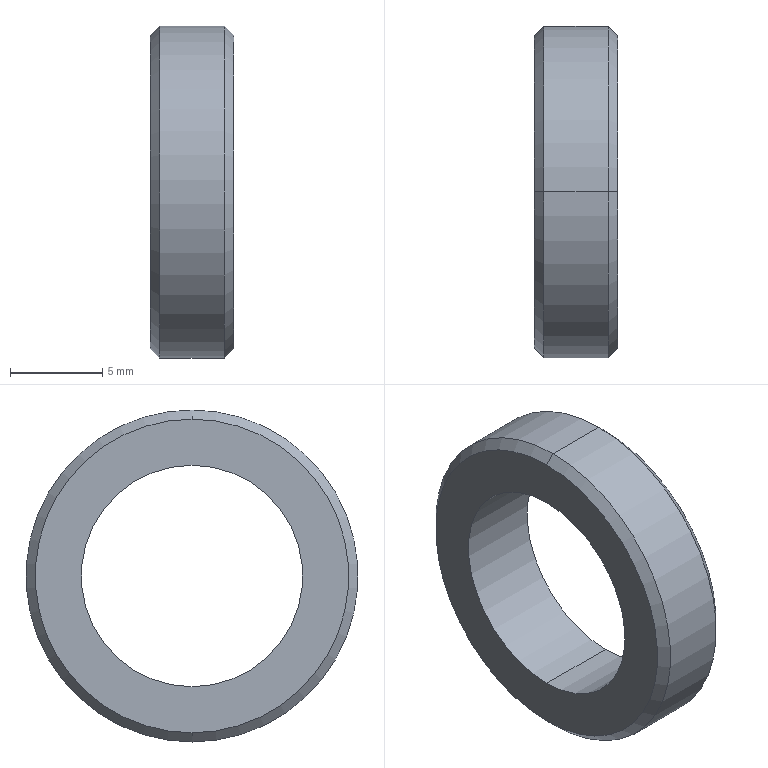Part | STEP file | 0245_008_CLBUM12-18-4.5 | 1 solid | 10 faces | box 4.5 x 18 x 18 mm | volume 622.297 mm3 | cone 4 | cylinder 4 | plane 2 | commonest cylinder face diameters 12 x2 18 x2
STEP:
#1=CARTESIAN_POINT('',(0.,0.,0.));
#2=DIRECTION('',(0.,0.,1.));
#3=DIRECTION('',(1.,0.,0.));
#4=AXIS2_PLACEMENT_3D('',#1,#2,#3);
#5=CARTESIAN_POINT('',(0.,0.,8.5));
#6=VERTEX_POINT('',#5);
#7=CARTESIAN_POINT('',(0.,0.,-8.5));
#8=VERTEX_POINT('',#7);
#9=CARTESIAN_POINT('',(0.,0.,0.));
#10=DIRECTION('',(-1.,0.,0.));
#11=DIRECTION('',(0.,0.,-1.));
#12=AXIS2_PLACEMENT_3D('',#9,#10,#11);
#13=CIRCLE('',#12,8.5);
#14=CARTESIAN_POINT('',(0.5,0.,0.));
#15=DIRECTION('',(1.,0.,0.));
#16=DIRECTION('',(0.,0.,-1.));
#17=AXIS2_PLACEMENT_3D('',#14,#15,#16);
#18=CONICAL_SURFACE('',#17,9.,0.7854);
#19=CARTESIAN_POINT('',(6.283,-0.5));
#20=DIRECTION('',(-1.,0.));
#21=VECTOR('',#20,1.);
#22=LINE('',#19,#21);
#23=(GEOMETRIC_REPRESENTATION_CONTEXT(2)PARAMETRIC_REPRESENTATION_CONTEXT()REPRESENTATION_CONTEXT('',''));
#24=DEFINITIONAL_REPRESENTATION('',(#22),#23);
#25=PCURVE('',#18,#24);
#26=CARTESIAN_POINT('',(0.,7.25,0.));
#27=DIRECTION('',(-1.,0.,0.));
#28=DIRECTION('',(0.,0.,1.));
#29=AXIS2_PLACEMENT_3D('',#26,#27,#28);
#30=PLANE('',#29);
#31=CARTESIAN_POINT('',(0.,-7.25));
#32=DIRECTION('',(-1.,0.));
#33=AXIS2_PLACEMENT_2D('',#31,#32);
#34=CIRCLE('',#33,8.5);
#35=(GEOMETRIC_REPRESENTATION_CONTEXT(2)PARAMETRIC_REPRESENTATION_CONTEXT()REPRESENTATION_CONTEXT('',''));
#36=DEFINITIONAL_REPRESENTATION('',(#34),#35);
#37=PCURVE('',#30,#36);
#38=SURFACE_CURVE('',#13,(#25,#37),.PCURVE_S1.);
#39=EDGE_CURVE('',#6,#8,#38,.T.);
#40=ORIENTED_EDGE('',*,*,#39,.F.);
#41=CARTESIAN_POINT('',(0.5,0.,9.));
#42=VERTEX_POINT('',#41);
#43=CARTESIAN_POINT('',(0.5,0.,9.));
#44=DIRECTION('',(0.7071,0.,0.7071));
#45=VECTOR('',#44,1.);
#46=LINE('',#43,#45);
#47=CARTESIAN_POINT('',(3.142,0.));
#48=DIRECTION('',(0.,1.));
#49=VECTOR('',#48,1.);
#50=LINE('',#47,#49);
#51=(GEOMETRIC_REPRESENTATION_CONTEXT(2)PARAMETRIC_REPRESENTATION_CONTEXT()REPRESENTATION_CONTEXT('',''));
#52=DEFINITIONAL_REPRESENTATION('',(#50),#51);
#53=PCURVE('',#18,#52);
#54=CARTESIAN_POINT('',(0.5,0.,0.));
#55=DIRECTION('',(1.,0.,0.));
#56=DIRECTION('',(0.,0.,-1.));
#57=AXIS2_PLACEMENT_3D('',#54,#55,#56);
#58=CONICAL_SURFACE('',#57,9.,0.7854);
#59=CARTESIAN_POINT('',(3.142,0.));
#60=DIRECTION('',(0.,1.));
#61=VECTOR('',#60,1.);
#62=LINE('',#59,#61);
#63=(GEOMETRIC_REPRESENTATION_CONTEXT(2)PARAMETRIC_REPRESENTATION_CONTEXT()REPRESENTATION_CONTEXT('',''));
#64=DEFINITIONAL_REPRESENTATION('',(#62),#63);
#65=PCURVE('',#58,#64);
#66=SURFACE_CURVE('',#46,(#53,#65),.PCURVE_S1.);
#67=EDGE_CURVE('',#6,#42,#66,.T.);
#68=ORIENTED_EDGE('',*,*,#67,.T.);
#69=CARTESIAN_POINT('',(0.5,0.,-9.));
#70=VERTEX_POINT('',#69);
#71=CARTESIAN_POINT('',(0.5,0.,0.));
#72=DIRECTION('',(-1.,0.,0.));
#73=DIRECTION('',(0.,1.,0.));
#74=AXIS2_PLACEMENT_3D('',#71,#72,#73);
#75=CIRCLE('',#74,9.);
#76=CARTESIAN_POINT('',(7.854,0.));
#77=DIRECTION('',(-1.,0.));
#78=VECTOR('',#77,1.);
#79=LINE('',#76,#78);
#80=(GEOMETRIC_REPRESENTATION_CONTEXT(2)PARAMETRIC_REPRESENTATION_CONTEXT()REPRESENTATION_CONTEXT('',''));
#81=DEFINITIONAL_REPRESENTATION('',(#79),#80);
#82=PCURVE('',#18,#81);
#83=CARTESIAN_POINT('',(2.25,0.,0.));
#84=DIRECTION('',(1.,0.,0.));
#85=DIRECTION('',(0.,0.,-1.));
#86=AXIS2_PLACEMENT_3D('',#83,#84,#85);
#87=CYLINDRICAL_SURFACE('',#86,9.);
#88=CARTESIAN_POINT('',(7.854,-1.75));
#89=DIRECTION('',(-1.,0.));
#90=VECTOR('',#89,1.);
#91=LINE('',#88,#90);
#92=(GEOMETRIC_REPRESENTATION_CONTEXT(2)PARAMETRIC_REPRESENTATION_CONTEXT()REPRESENTATION_CONTEXT('',''));
#93=DEFINITIONAL_REPRESENTATION('',(#91),#92);
#94=PCURVE('',#87,#93);
#95=SURFACE_CURVE('',#75,(#82,#94),.PCURVE_S1.);
#96=EDGE_CURVE('',#42,#70,#95,.T.);
#97=ORIENTED_EDGE('',*,*,#96,.T.);
#98=CARTESIAN_POINT('',(0.5,0.,-9.));
#99=DIRECTION('',(0.7071,0.,-0.7071));
#100=VECTOR('',#99,1.);
#101=LINE('',#98,#100);
#102=CARTESIAN_POINT('',(0.,0.));
#103=DIRECTION('',(0.,1.));
#104=VECTOR('',#103,1.);
#105=LINE('',#102,#104);
#106=(GEOMETRIC_REPRESENTATION_CONTEXT(2)PARAMETRIC_REPRESENTATION_CONTEXT()REPRESENTATION_CONTEXT('',''));
#107=DEFINITIONAL_REPRESENTATION('',(#105),#106);
#108=PCURVE('',#18,#107);
#109=CARTESIAN_POINT('',(6.283,0.));
#110=DIRECTION('',(0.,1.));
#111=VECTOR('',#110,1.);
#112=LINE('',#109,#111);
#113=(GEOMETRIC_REPRESENTATION_CONTEXT(2)PARAMETRIC_REPRESENTATION_CONTEXT()REPRESENTATION_CONTEXT('',''));
#114=DEFINITIONAL_REPRESENTATION('',(#112),#113);
#115=PCURVE('',#58,#114);
#116=SURFACE_CURVE('',#101,(#108,#115),.PCURVE_S1.);
#117=EDGE_CURVE('',#8,#70,#116,.T.);
#118=ORIENTED_EDGE('',*,*,#117,.F.);
#119=EDGE_LOOP('',(#40,#68,#97,#118));
#120=FACE_BOUND('',#119,.T.);
#121=ADVANCED_FACE('',(#120),#18,.T.);
#122=CARTESIAN_POINT('',(0.,0.,-6.));
#123=VERTEX_POINT('',#122);
#124=CARTESIAN_POINT('',(4.5,0.,-6.));
#125=VERTEX_POINT('',#124);
#126=CARTESIAN_POINT('',(2.25,0.,-6.));
#127=DIRECTION('',(1.,0.,0.));
#128=VECTOR('',#127,1.);
#129=LINE('',#126,#128);
#130=CARTESIAN_POINT('',(2.25,0.,0.));
#131=DIRECTION('',(1.,0.,0.));
#132=DIRECTION('',(0.,0.,-1.));
#133=AXIS2_PLACEMENT_3D('',#130,#131,#132);
#134=CYLINDRICAL_SURFACE('',#133,6.);
#135=CARTESIAN_POINT('',(6.283,0.));
#136=DIRECTION('',(0.,1.));
#137=VECTOR('',#136,1.);
#138=LINE('',#135,#137);
#139=(GEOMETRIC_REPRESENTATION_CONTEXT(2)PARAMETRIC_REPRESENTATION_CONTEXT()REPRESENTATION_CONTEXT('',''));
#140=DEFINITIONAL_REPRESENTATION('',(#138),#139);
#141=PCURVE('',#134,#140);
#142=CARTESIAN_POINT('',(2.25,0.,0.));
#143=DIRECTION('',(1.,0.,0.));
#144=DIRECTION('',(0.,0.,-1.));
#145=AXIS2_PLACEMENT_3D('',#142,#143,#144);
#146=CYLINDRICAL_SURFACE('',#145,6.);
#147=CARTESIAN_POINT('',(0.,0.));
#148=DIRECTION('',(0.,1.));
#149=VECTOR('',#148,1.);
#150=LINE('',#147,#149);
#151=(GEOMETRIC_REPRESENTATION_CONTEXT(2)PARAMETRIC_REPRESENTATION_CONTEXT()REPRESENTATION_CONTEXT('',''));
#152=DEFINITIONAL_REPRESENTATION('',(#150),#151);
#153=PCURVE('',#146,#152);
#154=SURFACE_CURVE('',#129,(#141,#153),.PCURVE_S1.);
#155=EDGE_CURVE('',#123,#125,#154,.T.);
#156=ORIENTED_EDGE('',*,*,#155,.T.);
#157=CARTESIAN_POINT('',(4.5,0.,6.));
#158=VERTEX_POINT('',#157);
#159=CARTESIAN_POINT('',(4.5,0.,0.));
#160=DIRECTION('',(-1.,0.,0.));
#161=DIRECTION('',(0.,0.,-1.));
#162=AXIS2_PLACEMENT_3D('',#159,#160,#161);
#163=CIRCLE('',#162,6.);
#164=CARTESIAN_POINT('',(6.283,2.25));
#165=DIRECTION('',(-1.,0.));
#166=VECTOR('',#165,1.);
#167=LINE('',#164,#166);
#168=(GEOMETRIC_REPRESENTATION_CONTEXT(2)PARAMETRIC_REPRESENTATION_CONTEXT()REPRESENTATION_CONTEXT('',''));
#169=DEFINITIONAL_REPRESENTATION('',(#167),#168);
#170=PCURVE('',#134,#169);
#171=CARTESIAN_POINT('',(4.5,7.25,0.));
#172=DIRECTION('',(1.,0.,0.));
#173=DIRECTION('',(0.,0.,-1.));
#174=AXIS2_PLACEMENT_3D('',#171,#172,#173);
#175=PLANE('',#174);
#176=CARTESIAN_POINT('',(6.,-7.25));
#177=CARTESIAN_POINT('',(6.,-17.642));
#178=CARTESIAN_POINT('',(-3.,-12.446));
#179=CARTESIAN_POINT('',(-12.,-7.25));
#180=CARTESIAN_POINT('',(-3.,-2.054));
#181=CARTESIAN_POINT('',(6.,3.142));
#182=CARTESIAN_POINT('',(6.,-7.25));
#183=(BOUNDED_CURVE()B_SPLINE_CURVE(2,(#176,#177,#178,#179,#180,#181,#182),.UNSPECIFIED.,.T.,.F.)B_SPLINE_CURVE_WITH_KNOTS((1,2,2,2,2,1),(-2.094,0.,2.094,4.189,6.283,8.378),.UNSPECIFIED.)CURVE()GEOMETRIC_REPRESENTATION_ITEM()RATIONAL_B_SPLINE_CURVE((1.,0.5,1.,0.5,1.,0.5,1.))REPRESENTATION_ITEM(''));
#184=(GEOMETRIC_REPRESENTATION_CONTEXT(2)PARAMETRIC_REPRESENTATION_CONTEXT()REPRESENTATION_CONTEXT('',''));
#185=DEFINITIONAL_REPRESENTATION('',(#183),#184);
#186=PCURVE('',#175,#185);
#187=SURFACE_CURVE('',#163,(#170,#186),.PCURVE_S1.);
#188=EDGE_CURVE('',#125,#158,#187,.T.);
#189=ORIENTED_EDGE('',*,*,#188,.T.);
#190=CARTESIAN_POINT('',(0.,0.,6.));
#191=VERTEX_POINT('',#190);
#192=CARTESIAN_POINT('',(2.25,0.,6.));
#193=DIRECTION('',(1.,0.,0.));
#194=VECTOR('',#193,1.);
#195=LINE('',#192,#194);
#196=CARTESIAN_POINT('',(3.142,0.));
#197=DIRECTION('',(0.,1.));
#198=VECTOR('',#197,1.);
#199=LINE('',#196,#198);
#200=(GEOMETRIC_REPRESENTATION_CONTEXT(2)PARAMETRIC_REPRESENTATION_CONTEXT()REPRESENTATION_CONTEXT('',''));
#201=DEFINITIONAL_REPRESENTATION('',(#199),#200);
#202=PCURVE('',#134,#201);
#203=CARTESIAN_POINT('',(3.142,0.));
#204=DIRECTION('',(0.,1.));
#205=VECTOR('',#204,1.);
#206=LINE('',#203,#205);
#207=(GEOMETRIC_REPRESENTATION_CONTEXT(2)PARAMETRIC_REPRESENTATION_CONTEXT()REPRESENTATION_CONTEXT('',''));
#208=DEFINITIONAL_REPRESENTATION('',(#206),#207);
#209=PCURVE('',#146,#208);
#210=SURFACE_CURVE('',#195,(#202,#209),.PCURVE_S1.);
#211=EDGE_CURVE('',#191,#158,#210,.T.);
#212=ORIENTED_EDGE('',*,*,#211,.F.);
#213=CARTESIAN_POINT('',(0.,0.,0.));
#214=DIRECTION('',(1.,0.,0.));
#215=DIRECTION('',(0.,0.,-1.));
#216=AXIS2_PLACEMENT_3D('',#213,#214,#215);
#217=CIRCLE('',#216,6.);
#218=CARTESIAN_POINT('',(0.,-2.25));
#219=DIRECTION('',(1.,0.));
#220=VECTOR('',#219,1.);
#221=LINE('',#218,#220);
#222=(GEOMETRIC_REPRESENTATION_CONTEXT(2)PARAMETRIC_REPRESENTATION_CONTEXT()REPRESENTATION_CONTEXT('',''));
#223=DEFINITIONAL_REPRESENTATION('',(#221),#222);
#224=PCURVE('',#134,#223);
#225=CARTESIAN_POINT('',(-6.,-7.25));
#226=CARTESIAN_POINT('',(-6.,3.142));
#227=CARTESIAN_POINT('',(3.,-2.054));
#228=CARTESIAN_POINT('',(12.,-7.25));
#229=CARTESIAN_POINT('',(3.,-12.446));
#230=CARTESIAN_POINT('',(-6.,-17.642));
#231=CARTESIAN_POINT('',(-6.,-7.25));
#232=(BOUNDED_CURVE()B_SPLINE_CURVE(2,(#225,#226,#227,#228,#229,#230,#231),.UNSPECIFIED.,.T.,.F.)B_SPLINE_CURVE_WITH_KNOTS((1,2,2,2,2,1),(-2.094,0.,2.094,4.189,6.283,8.378),.UNSPECIFIED.)CURVE()GEOMETRIC_REPRESENTATION_ITEM()RATIONAL_B_SPLINE_CURVE((1.,0.5,1.,0.5,1.,0.5,1.))REPRESENTATION_ITEM(''));
#233=(GEOMETRIC_REPRESENTATION_CONTEXT(2)PARAMETRIC_REPRESENTATION_CONTEXT()REPRESENTATION_CONTEXT('',''));
#234=DEFINITIONAL_REPRESENTATION('',(#232),#233);
#235=PCURVE('',#30,#234);
#236=SURFACE_CURVE('',#217,(#224,#235),.PCURVE_S1.);
#237=EDGE_CURVE('',#191,#123,#236,.T.);
#238=ORIENTED_EDGE('',*,*,#237,.T.);
#239=EDGE_LOOP('',(#156,#189,#212,#238));
#240=FACE_BOUND('',#239,.F.);
#241=ADVANCED_FACE('',(#240),#134,.F.);
#242=ORIENTED_EDGE('',*,*,#96,.F.);
#243=CARTESIAN_POINT('',(4.,0.,9.));
#244=VERTEX_POINT('',#243);
#245=CARTESIAN_POINT('',(2.25,0.,9.));
#246=DIRECTION('',(1.,0.,0.));
#247=VECTOR('',#246,1.);
#248=LINE('',#245,#247);
#249=CARTESIAN_POINT('',(3.142,0.));
#250=DIRECTION('',(0.,1.));
#251=VECTOR('',#250,1.);
#252=LINE('',#249,#251);
#253=(GEOMETRIC_REPRESENTATION_CONTEXT(2)PARAMETRIC_REPRESENTATION_CONTEXT()REPRESENTATION_CONTEXT('',''));
#254=DEFINITIONAL_REPRESENTATION('',(#252),#253);
#255=PCURVE('',#87,#254);
#256=CARTESIAN_POINT('',(2.25,0.,0.));
#257=DIRECTION('',(1.,0.,0.));
#258=DIRECTION('',(0.,0.,-1.));
#259=AXIS2_PLACEMENT_3D('',#256,#257,#258);
#260=CYLINDRICAL_SURFACE('',#259,9.);
#261=CARTESIAN_POINT('',(3.142,0.));
#262=DIRECTION('',(0.,1.));
#263=VECTOR('',#262,1.);
#264=LINE('',#261,#263);
#265=(GEOMETRIC_REPRESENTATION_CONTEXT(2)PARAMETRIC_REPRESENTATION_CONTEXT()REPRESENTATION_CONTEXT('',''));
#266=DEFINITIONAL_REPRESENTATION('',(#264),#265);
#267=PCURVE('',#260,#266);
#268=SURFACE_CURVE('',#248,(#255,#267),.PCURVE_S1.);
#269=EDGE_CURVE('',#42,#244,#268,.T.);
#270=ORIENTED_EDGE('',*,*,#269,.T.);
#271=CARTESIAN_POINT('',(4.,0.,-9.));
#272=VERTEX_POINT('',#271);
#273=CARTESIAN_POINT('',(4.,0.,0.));
#274=DIRECTION('',(-1.,0.,0.));
#275=DIRECTION('',(0.,0.,-1.));
#276=AXIS2_PLACEMENT_3D('',#273,#274,#275);
#277=CIRCLE('',#276,9.);
#278=CARTESIAN_POINT('',(6.283,1.75));
#279=DIRECTION('',(-1.,0.));
#280=VECTOR('',#279,1.);
#281=LINE('',#278,#280);
#282=(GEOMETRIC_REPRESENTATION_CONTEXT(2)PARAMETRIC_REPRESENTATION_CONTEXT()REPRESENTATION_CONTEXT('',''));
#283=DEFINITIONAL_REPRESENTATION('',(#281),#282);
#284=PCURVE('',#87,#283);
#285=CARTESIAN_POINT('',(4.,0.,0.));
#286=DIRECTION('',(-1.,0.,0.));
#287=DIRECTION('',(0.,0.,1.));
#288=AXIS2_PLACEMENT_3D('',#285,#286,#287);
#289=CONICAL_SURFACE('',#288,9.,0.7854);
#290=CARTESIAN_POINT('',(-3.142,0.));
#291=DIRECTION('',(1.,0.));
#292=VECTOR('',#291,1.);
#293=LINE('',#290,#292);
#294=(GEOMETRIC_REPRESENTATION_CONTEXT(2)PARAMETRIC_REPRESENTATION_CONTEXT()REPRESENTATION_CONTEXT('',''));
#295=DEFINITIONAL_REPRESENTATION('',(#293),#294);
#296=PCURVE('',#289,#295);
#297=SURFACE_CURVE('',#277,(#284,#296),.PCURVE_S1.);
#298=EDGE_CURVE('',#244,#272,#297,.T.);
#299=ORIENTED_EDGE('',*,*,#298,.T.);
#300=CARTESIAN_POINT('',(2.25,0.,-9.));
#301=DIRECTION('',(1.,0.,0.));
#302=VECTOR('',#301,1.);
#303=LINE('',#300,#302);
#304=CARTESIAN_POINT('',(0.,0.));
#305=DIRECTION('',(0.,1.));
#306=VECTOR('',#305,1.);
#307=LINE('',#304,#306);
#308=(GEOMETRIC_REPRESENTATION_CONTEXT(2)PARAMETRIC_REPRESENTATION_CONTEXT()REPRESENTATION_CONTEXT('',''));
#309=DEFINITIONAL_REPRESENTATION('',(#307),#308);
#310=PCURVE('',#87,#309);
#311=CARTESIAN_POINT('',(6.283,0.));
#312=DIRECTION('',(0.,1.));
#313=VECTOR('',#312,1.);
#314=LINE('',#311,#313);
#315=(GEOMETRIC_REPRESENTATION_CONTEXT(2)PARAMETRIC_REPRESENTATION_CONTEXT()REPRESENTATION_CONTEXT('',''));
#316=DEFINITIONAL_REPRESENTATION('',(#314),#315);
#317=PCURVE('',#260,#316);
#318=SURFACE_CURVE('',#303,(#310,#317),.PCURVE_S1.);
#319=EDGE_CURVE('',#70,#272,#318,.T.);
#320=ORIENTED_EDGE('',*,*,#319,.F.);
#321=EDGE_LOOP('',(#242,#270,#299,#320));
#322=FACE_BOUND('',#321,.T.);
#323=ADVANCED_FACE('',(#322),#87,.T.);
#324=CARTESIAN_POINT('',(4.5,0.,-8.5));
#325=VERTEX_POINT('',#324);
#326=CARTESIAN_POINT('',(4.5,0.,8.5));
#327=VERTEX_POINT('',#326);
#328=CARTESIAN_POINT('',(4.5,0.,0.));
#329=DIRECTION('',(1.,0.,0.));
#330=DIRECTION('',(0.,0.,1.));
#331=AXIS2_PLACEMENT_3D('',#328,#329,#330);
#332=CIRCLE('',#331,8.5);
#333=CARTESIAN_POINT('',(6.283,-0.5));
#334=DIRECTION('',(-1.,0.));
#335=VECTOR('',#334,1.);
#336=LINE('',#333,#335);
#337=(GEOMETRIC_REPRESENTATION_CONTEXT(2)PARAMETRIC_REPRESENTATION_CONTEXT()REPRESENTATION_CONTEXT('',''));
#338=DEFINITIONAL_REPRESENTATION('',(#336),#337);
#339=PCURVE('',#289,#338);
#340=CARTESIAN_POINT('',(0.,-7.25));
#341=DIRECTION('',(-1.,0.));
#342=AXIS2_PLACEMENT_2D('',#340,#341);
#343=CIRCLE('',#342,8.5);
#344=(GEOMETRIC_REPRESENTATION_CONTEXT(2)PARAMETRIC_REPRESENTATION_CONTEXT()REPRESENTATION_CONTEXT('',''));
#345=DEFINITIONAL_REPRESENTATION('',(#343),#344);
#346=PCURVE('',#175,#345);
#347=SURFACE_CURVE('',#332,(#339,#346),.PCURVE_S1.);
#348=EDGE_CURVE('',#325,#327,#347,.T.);
#349=ORIENTED_EDGE('',*,*,#348,.F.);
#350=CARTESIAN_POINT('',(4.,0.,-9.));
#351=DIRECTION('',(-0.7071,0.,-0.7071));
#352=VECTOR('',#351,1.);
#353=LINE('',#350,#352);
#354=CARTESIAN_POINT('',(3.142,0.));
#355=DIRECTION('',(0.,1.));
#356=VECTOR('',#355,1.);
#357=LINE('',#354,#356);
#358=(GEOMETRIC_REPRESENTATION_CONTEXT(2)PARAMETRIC_REPRESENTATION_CONTEXT()REPRESENTATION_CONTEXT('',''));
#359=DEFINITIONAL_REPRESENTATION('',(#357),#358);
#360=PCURVE('',#289,#359);
#361=CARTESIAN_POINT('',(4.,0.,0.));
#362=DIRECTION('',(-1.,0.,0.));
#363=DIRECTION('',(0.,0.,1.));
#364=AXIS2_PLACEMENT_3D('',#361,#362,#363);
#365=CONICAL_SURFACE('',#364,9.,0.7854);
#366=CARTESIAN_POINT('',(3.142,0.));
#367=DIRECTION('',(0.,1.));
#368=VECTOR('',#367,1.);
#369=LINE('',#366,#368);
#370=(GEOMETRIC_REPRESENTATION_CONTEXT(2)PARAMETRIC_REPRESENTATION_CONTEXT()REPRESENTATION_CONTEXT('',''));
#371=DEFINITIONAL_REPRESENTATION('',(#369),#370);
#372=PCURVE('',#365,#371);
#373=SURFACE_CURVE('',#353,(#360,#372),.PCURVE_S1.);
#374=EDGE_CURVE('',#325,#272,#373,.T.);
#375=ORIENTED_EDGE('',*,*,#374,.T.);
#376=ORIENTED_EDGE('',*,*,#298,.F.);
#377=CARTESIAN_POINT('',(4.,0.,9.));
#378=DIRECTION('',(-0.7071,0.,0.7071));
#379=VECTOR('',#378,1.);
#380=LINE('',#377,#379);
#381=CARTESIAN_POINT('',(0.,0.));
#382=DIRECTION('',(0.,1.));
#383=VECTOR('',#382,1.);
#384=LINE('',#381,#383);
#385=(GEOMETRIC_REPRESENTATION_CONTEXT(2)PARAMETRIC_REPRESENTATION_CONTEXT()REPRESENTATION_CONTEXT('',''));
#386=DEFINITIONAL_REPRESENTATION('',(#384),#385);
#387=PCURVE('',#289,#386);
#388=CARTESIAN_POINT('',(6.283,0.));
#389=DIRECTION('',(0.,1.));
#390=VECTOR('',#389,1.);
#391=LINE('',#388,#390);
#392=(GEOMETRIC_REPRESENTATION_CONTEXT(2)PARAMETRIC_REPRESENTATION_CONTEXT()REPRESENTATION_CONTEXT('',''));
#393=DEFINITIONAL_REPRESENTATION('',(#391),#392);
#394=PCURVE('',#365,#393);
#395=SURFACE_CURVE('',#380,(#387,#394),.PCURVE_S1.);
#396=EDGE_CURVE('',#327,#244,#395,.T.);
#397=ORIENTED_EDGE('',*,*,#396,.F.);
#398=EDGE_LOOP('',(#349,#375,#376,#397));
#399=FACE_BOUND('',#398,.T.);
#400=ADVANCED_FACE('',(#399),#289,.T.);
#401=CARTESIAN_POINT('',(0.,0.,0.));
#402=DIRECTION('',(-1.,0.,0.));
#403=DIRECTION('',(0.,0.,-1.));
#404=AXIS2_PLACEMENT_3D('',#401,#402,#403);
#405=CIRCLE('',#404,8.5);
#406=CARTESIAN_POINT('',(0.,-7.25));
#407=DIRECTION('',(-1.,0.));
#408=AXIS2_PLACEMENT_2D('',#406,#407);
#409=CIRCLE('',#408,8.5);
#410=(GEOMETRIC_REPRESENTATION_CONTEXT(2)PARAMETRIC_REPRESENTATION_CONTEXT()REPRESENTATION_CONTEXT('',''));
#411=DEFINITIONAL_REPRESENTATION('',(#409),#410);
#412=PCURVE('',#30,#411);
#413=CARTESIAN_POINT('',(6.283,-0.5));
#414=DIRECTION('',(-1.,0.));
#415=VECTOR('',#414,1.);
#416=LINE('',#413,#415);
#417=(GEOMETRIC_REPRESENTATION_CONTEXT(2)PARAMETRIC_REPRESENTATION_CONTEXT()REPRESENTATION_CONTEXT('',''));
#418=DEFINITIONAL_REPRESENTATION('',(#416),#417);
#419=PCURVE('',#58,#418);
#420=SURFACE_CURVE('',#405,(#412,#419),.PCURVE_S1.);
#421=EDGE_CURVE('',#8,#6,#420,.T.);
#422=ORIENTED_EDGE('',*,*,#421,.T.);
#423=ORIENTED_EDGE('',*,*,#39,.T.);
#424=EDGE_LOOP('',(#422,#423));
#425=FACE_BOUND('',#424,.T.);
#426=CARTESIAN_POINT('',(0.,0.,0.));
#427=DIRECTION('',(1.,0.,0.));
#428=DIRECTION('',(0.,0.,-1.));
#429=AXIS2_PLACEMENT_3D('',#426,#427,#428);
#430=CIRCLE('',#429,6.);
#431=CARTESIAN_POINT('',(-6.,-7.25));
#432=CARTESIAN_POINT('',(-6.,3.142));
#433=CARTESIAN_POINT('',(3.,-2.054));
#434=CARTESIAN_POINT('',(12.,-7.25));
#435=CARTESIAN_POINT('',(3.,-12.446));
#436=CARTESIAN_POINT('',(-6.,-17.642));
#437=CARTESIAN_POINT('',(-6.,-7.25));
#438=(BOUNDED_CURVE()B_SPLINE_CURVE(2,(#431,#432,#433,#434,#435,#436,#437),.UNSPECIFIED.,.T.,.F.)B_SPLINE_CURVE_WITH_KNOTS((1,2,2,2,2,1),(-2.094,0.,2.094,4.189,6.283,8.378),.UNSPECIFIED.)CURVE()GEOMETRIC_REPRESENTATION_ITEM()RATIONAL_B_SPLINE_CURVE((1.,0.5,1.,0.5,1.,0.5,1.))REPRESENTATION_ITEM(''));
#439=(GEOMETRIC_REPRESENTATION_CONTEXT(2)PARAMETRIC_REPRESENTATION_CONTEXT()REPRESENTATION_CONTEXT('',''));
#440=DEFINITIONAL_REPRESENTATION('',(#438),#439);
#441=PCURVE('',#30,#440);
#442=CARTESIAN_POINT('',(0.,-2.25));
#443=DIRECTION('',(1.,0.));
#444=VECTOR('',#443,1.);
#445=LINE('',#442,#444);
#446=(GEOMETRIC_REPRESENTATION_CONTEXT(2)PARAMETRIC_REPRESENTATION_CONTEXT()REPRESENTATION_CONTEXT('',''));
#447=DEFINITIONAL_REPRESENTATION('',(#445),#446);
#448=PCURVE('',#146,#447);
#449=SURFACE_CURVE('',#430,(#441,#448),.PCURVE_S1.);
#450=EDGE_CURVE('',#123,#191,#449,.T.);
#451=ORIENTED_EDGE('',*,*,#450,.T.);
#452=ORIENTED_EDGE('',*,*,#237,.T.);
#453=EDGE_LOOP('',(#451,#452));
#454=FACE_BOUND('',#453,.T.);
#455=ADVANCED_FACE('',(#425,#454),#30,.T.);
#456=ORIENTED_EDGE('',*,*,#67,.F.);
#457=ORIENTED_EDGE('',*,*,#421,.F.);
#458=ORIENTED_EDGE('',*,*,#117,.T.);
#459=CARTESIAN_POINT('',(0.5,0.,0.));
#460=DIRECTION('',(-1.,0.,0.));
#461=DIRECTION('',(0.,1.,0.));
#462=AXIS2_PLACEMENT_3D('',#459,#460,#461);
#463=CIRCLE('',#462,9.);
#464=CARTESIAN_POINT('',(7.854,0.));
#465=DIRECTION('',(-1.,0.));
#466=VECTOR('',#465,1.);
#467=LINE('',#464,#466);
#468=(GEOMETRIC_REPRESENTATION_CONTEXT(2)PARAMETRIC_REPRESENTATION_CONTEXT()REPRESENTATION_CONTEXT('',''));
#469=DEFINITIONAL_REPRESENTATION('',(#467),#468);
#470=PCURVE('',#58,#469);
#471=CARTESIAN_POINT('',(7.854,-1.75));
#472=DIRECTION('',(-1.,0.));
#473=VECTOR('',#472,1.);
#474=LINE('',#471,#473);
#475=(GEOMETRIC_REPRESENTATION_CONTEXT(2)PARAMETRIC_REPRESENTATION_CONTEXT()REPRESENTATION_CONTEXT('',''));
#476=DEFINITIONAL_REPRESENTATION('',(#474),#475);
#477=PCURVE('',#260,#476);
#478=SURFACE_CURVE('',#463,(#470,#477),.PCURVE_S1.);
#479=EDGE_CURVE('',#70,#42,#478,.T.);
#480=ORIENTED_EDGE('',*,*,#479,.T.);
#481=EDGE_LOOP('',(#456,#457,#458,#480));
#482=FACE_BOUND('',#481,.T.);
#483=ADVANCED_FACE('',(#482),#58,.T.);
#484=CARTESIAN_POINT('',(4.5,0.,0.));
#485=DIRECTION('',(-1.,0.,0.));
#486=DIRECTION('',(0.,0.,-1.));
#487=AXIS2_PLACEMENT_3D('',#484,#485,#486);
#488=CIRCLE('',#487,6.);
#489=CARTESIAN_POINT('',(6.283,2.25));
#490=DIRECTION('',(-1.,0.));
#491=VECTOR('',#490,1.);
#492=LINE('',#489,#491);
#493=(GEOMETRIC_REPRESENTATION_CONTEXT(2)PARAMETRIC_REPRESENTATION_CONTEXT()REPRESENTATION_CONTEXT('',''));
#494=DEFINITIONAL_REPRESENTATION('',(#492),#493);
#495=PCURVE('',#146,#494);
#496=CARTESIAN_POINT('',(6.,-7.25));
#497=CARTESIAN_POINT('',(6.,-17.642));
#498=CARTESIAN_POINT('',(-3.,-12.446));
#499=CARTESIAN_POINT('',(-12.,-7.25));
#500=CARTESIAN_POINT('',(-3.,-2.054));
#501=CARTESIAN_POINT('',(6.,3.142));
#502=CARTESIAN_POINT('',(6.,-7.25));
#503=(BOUNDED_CURVE()B_SPLINE_CURVE(2,(#496,#497,#498,#499,#500,#501,#502),.UNSPECIFIED.,.T.,.F.)B_SPLINE_CURVE_WITH_KNOTS((1,2,2,2,2,1),(-2.094,0.,2.094,4.189,6.283,8.378),.UNSPECIFIED.)CURVE()GEOMETRIC_REPRESENTATION_ITEM()RATIONAL_B_SPLINE_CURVE((1.,0.5,1.,0.5,1.,0.5,1.))REPRESENTATION_ITEM(''));
#504=(GEOMETRIC_REPRESENTATION_CONTEXT(2)PARAMETRIC_REPRESENTATION_CONTEXT()REPRESENTATION_CONTEXT('',''));
#505=DEFINITIONAL_REPRESENTATION('',(#503),#504);
#506=PCURVE('',#175,#505);
#507=SURFACE_CURVE('',#488,(#495,#506),.PCURVE_S1.);
#508=EDGE_CURVE('',#158,#125,#507,.T.);
#509=ORIENTED_EDGE('',*,*,#508,.T.);
#510=ORIENTED_EDGE('',*,*,#155,.F.);
#511=ORIENTED_EDGE('',*,*,#450,.T.);
#512=ORIENTED_EDGE('',*,*,#211,.T.);
#513=EDGE_LOOP('',(#509,#510,#511,#512));
#514=FACE_BOUND('',#513,.F.);
#515=ADVANCED_FACE('',(#514),#146,.F.);
#516=ORIENTED_EDGE('',*,*,#269,.F.);
#517=ORIENTED_EDGE('',*,*,#479,.F.);
#518=ORIENTED_EDGE('',*,*,#319,.T.);
#519=CARTESIAN_POINT('',(4.,0.,0.));
#520=DIRECTION('',(-1.,0.,0.));
#521=DIRECTION('',(0.,0.,-1.));
#522=AXIS2_PLACEMENT_3D('',#519,#520,#521);
#523=CIRCLE('',#522,9.);
#524=CARTESIAN_POINT('',(6.283,1.75));
#525=DIRECTION('',(-1.,0.));
#526=VECTOR('',#525,1.);
#527=LINE('',#524,#526);
#528=(GEOMETRIC_REPRESENTATION_CONTEXT(2)PARAMETRIC_REPRESENTATION_CONTEXT()REPRESENTATION_CONTEXT('',''));
#529=DEFINITIONAL_REPRESENTATION('',(#527),#528);
#530=PCURVE('',#260,#529);
#531=CARTESIAN_POINT('',(3.142,0.));
#532=DIRECTION('',(1.,0.));
#533=VECTOR('',#532,1.);
#534=LINE('',#531,#533);
#535=(GEOMETRIC_REPRESENTATION_CONTEXT(2)PARAMETRIC_REPRESENTATION_CONTEXT()REPRESENTATION_CONTEXT('',''));
#536=DEFINITIONAL_REPRESENTATION('',(#534),#535);
#537=PCURVE('',#365,#536);
#538=SURFACE_CURVE('',#523,(#530,#537),.PCURVE_S1.);
#539=EDGE_CURVE('',#272,#244,#538,.T.);
#540=ORIENTED_EDGE('',*,*,#539,.T.);
#541=EDGE_LOOP('',(#516,#517,#518,#540));
#542=FACE_BOUND('',#541,.T.);
#543=ADVANCED_FACE('',(#542),#260,.T.);
#544=ORIENTED_EDGE('',*,*,#188,.T.);
#545=ORIENTED_EDGE('',*,*,#508,.T.);
#546=EDGE_LOOP('',(#544,#545));
#547=FACE_BOUND('',#546,.T.);
#548=CARTESIAN_POINT('',(4.5,0.,0.));
#549=DIRECTION('',(1.,0.,0.));
#550=DIRECTION('',(0.,0.,1.));
#551=AXIS2_PLACEMENT_3D('',#548,#549,#550);
#552=CIRCLE('',#551,8.5);
#553=CARTESIAN_POINT('',(0.,-7.25));
#554=DIRECTION('',(-1.,0.));
#555=AXIS2_PLACEMENT_2D('',#553,#554);
#556=CIRCLE('',#555,8.5);
#557=(GEOMETRIC_REPRESENTATION_CONTEXT(2)PARAMETRIC_REPRESENTATION_CONTEXT()REPRESENTATION_CONTEXT('',''));
#558=DEFINITIONAL_REPRESENTATION('',(#556),#557);
#559=PCURVE('',#175,#558);
#560=CARTESIAN_POINT('',(6.283,-0.5));
#561=DIRECTION('',(-1.,0.));
#562=VECTOR('',#561,1.);
#563=LINE('',#560,#562);
#564=(GEOMETRIC_REPRESENTATION_CONTEXT(2)PARAMETRIC_REPRESENTATION_CONTEXT()REPRESENTATION_CONTEXT('',''));
#565=DEFINITIONAL_REPRESENTATION('',(#563),#564);
#566=PCURVE('',#365,#565);
#567=SURFACE_CURVE('',#552,(#559,#566),.PCURVE_S1.);
#568=EDGE_CURVE('',#327,#325,#567,.T.);
#569=ORIENTED_EDGE('',*,*,#568,.T.);
#570=ORIENTED_EDGE('',*,*,#348,.T.);
#571=EDGE_LOOP('',(#569,#570));
#572=FACE_BOUND('',#571,.T.);
#573=ADVANCED_FACE('',(#547,#572),#175,.T.);
#574=ORIENTED_EDGE('',*,*,#374,.F.);
#575=ORIENTED_EDGE('',*,*,#568,.F.);
#576=ORIENTED_EDGE('',*,*,#396,.T.);
#577=ORIENTED_EDGE('',*,*,#539,.F.);
#578=EDGE_LOOP('',(#574,#575,#576,#577));
#579=FACE_BOUND('',#578,.T.);
#580=ADVANCED_FACE('',(#579),#365,.T.);
#581=CLOSED_SHELL('',(#121,#241,#323,#400,#455,#483,#515,#543,#573,#580));
#582=MANIFOLD_SOLID_BREP('',#581);
#583=(LENGTH_UNIT()NAMED_UNIT(*)SI_UNIT(.MILLI.,.METRE.));
#584=UNCERTAINTY_MEASURE_WITH_UNIT(LENGTH_MEASURE(0.0000001),#583,'','');
#585=(NAMED_UNIT(*)PLANE_ANGLE_UNIT()SI_UNIT($,.RADIAN.));
#586=(NAMED_UNIT(*)SI_UNIT($,.STERADIAN.)SOLID_ANGLE_UNIT());
#587=(GEOMETRIC_REPRESENTATION_CONTEXT(3)GLOBAL_UNCERTAINTY_ASSIGNED_CONTEXT((#584))GLOBAL_UNIT_ASSIGNED_CONTEXT((#583,#585,#586))REPRESENTATION_CONTEXT('',''));
#588=ADVANCED_BREP_SHAPE_REPRESENTATION('',(#4,#582),#587);